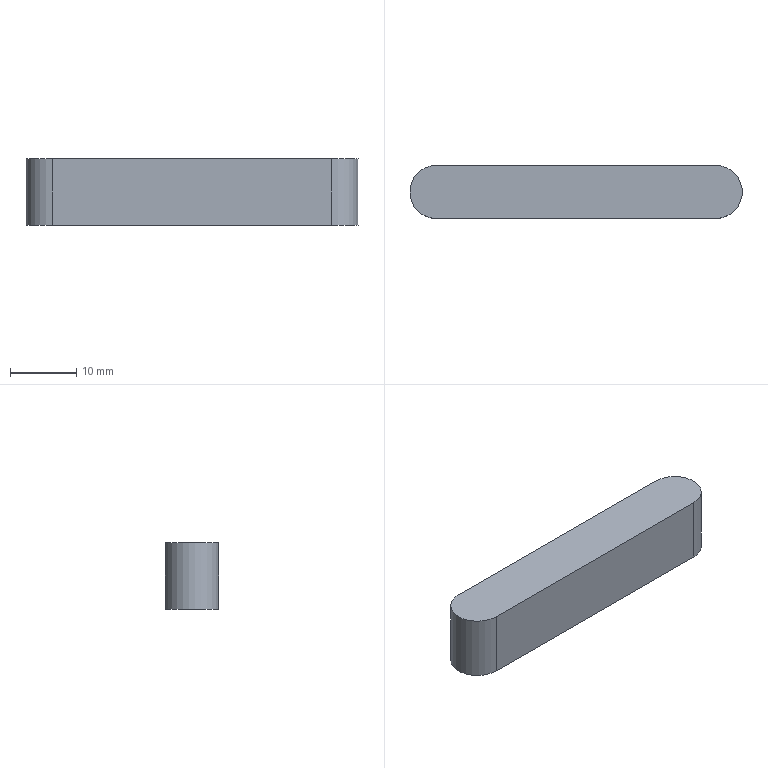Part | NX | features DATUM_CSYS 2, BLEND 1, EXTRUDE 1, SKETCH 1 | 1 solid | 6 faces | box 50 x 8 x 10 mm | volume 3863 mm3 | plane 4 | cylinder 2 | commonest cylinder face diameters 8 x2
STEP:
#1=CARTESIAN_POINT('',(-21.,-4.,10.));
#2=VERTEX_POINT('',#1);
#3=CARTESIAN_POINT('',(21.,-4.,10.));
#4=VERTEX_POINT('',#3);
#5=CARTESIAN_POINT('',(-25.,-4.,10.));
#6=DIRECTION('',(1.,0.,0.));
#7=VECTOR('',#6,1000.);
#8=LINE('',#5,#7);
#9=EDGE_CURVE('',#2,#4,#8,.T.);
#10=ORIENTED_EDGE('',*,*,#9,.F.);
#11=CARTESIAN_POINT('',(-21.,-4.,0.));
#12=VERTEX_POINT('',#11);
#13=CARTESIAN_POINT('',(-21.,-4.,10.));
#14=DIRECTION('',(0.,0.,-1.));
#15=VECTOR('',#14,1000.);
#16=LINE('',#13,#15);
#17=EDGE_CURVE('',#2,#12,#16,.T.);
#18=ORIENTED_EDGE('',*,*,#17,.T.);
#19=CARTESIAN_POINT('',(21.,-4.,0.));
#20=VERTEX_POINT('',#19);
#21=CARTESIAN_POINT('',(-25.,-4.,0.));
#22=DIRECTION('',(1.,0.,0.));
#23=VECTOR('',#22,1000.);
#24=LINE('',#21,#23);
#25=EDGE_CURVE('',#12,#20,#24,.T.);
#26=ORIENTED_EDGE('',*,*,#25,.T.);
#27=CARTESIAN_POINT('',(21.,-4.,10.));
#28=DIRECTION('',(0.,0.,-1.));
#29=VECTOR('',#28,1000.);
#30=LINE('',#27,#29);
#31=EDGE_CURVE('',#20,#4,#30,.F.);
#32=ORIENTED_EDGE('',*,*,#31,.T.);
#33=EDGE_LOOP('',(#10,#18,#26,#32));
#34=FACE_BOUND('',#33,.T.);
#35=CARTESIAN_POINT('',(-25.,-4.,10.));
#36=DIRECTION('',(0.,1.,0.));
#37=DIRECTION('',(0.,0.,1.));
#38=AXIS2_PLACEMENT_3D('',#35,#36,#37);
#39=PLANE('',#38);
#40=ADVANCED_FACE('',(#34),#39,.F.);
#41=CARTESIAN_POINT('',(21.,4.,0.));
#42=VERTEX_POINT('',#41);
#43=CARTESIAN_POINT('',(-21.,4.,0.));
#44=VERTEX_POINT('',#43);
#45=CARTESIAN_POINT('',(25.,4.,0.));
#46=DIRECTION('',(-1.,0.,0.));
#47=VECTOR('',#46,1000.);
#48=LINE('',#45,#47);
#49=EDGE_CURVE('',#42,#44,#48,.T.);
#50=ORIENTED_EDGE('',*,*,#49,.T.);
#51=CARTESIAN_POINT('',(-21.,4.,10.));
#52=VERTEX_POINT('',#51);
#53=CARTESIAN_POINT('',(-21.,4.,10.));
#54=DIRECTION('',(0.,0.,-1.));
#55=VECTOR('',#54,1000.);
#56=LINE('',#53,#55);
#57=EDGE_CURVE('',#44,#52,#56,.F.);
#58=ORIENTED_EDGE('',*,*,#57,.T.);
#59=CARTESIAN_POINT('',(21.,4.,10.));
#60=VERTEX_POINT('',#59);
#61=CARTESIAN_POINT('',(25.,4.,10.));
#62=DIRECTION('',(-1.,0.,0.));
#63=VECTOR('',#62,1000.);
#64=LINE('',#61,#63);
#65=EDGE_CURVE('',#60,#52,#64,.T.);
#66=ORIENTED_EDGE('',*,*,#65,.F.);
#67=CARTESIAN_POINT('',(21.,4.,10.));
#68=DIRECTION('',(0.,0.,-1.));
#69=VECTOR('',#68,1000.);
#70=LINE('',#67,#69);
#71=EDGE_CURVE('',#60,#42,#70,.T.);
#72=ORIENTED_EDGE('',*,*,#71,.T.);
#73=EDGE_LOOP('',(#50,#58,#66,#72));
#74=FACE_BOUND('',#73,.T.);
#75=CARTESIAN_POINT('',(25.,4.,10.));
#76=DIRECTION('',(0.,-1.,0.));
#77=DIRECTION('',(0.,0.,-1.));
#78=AXIS2_PLACEMENT_3D('',#75,#76,#77);
#79=PLANE('',#78);
#80=ADVANCED_FACE('',(#74),#79,.F.);
#81=ORIENTED_EDGE('',*,*,#65,.T.);
#82=CARTESIAN_POINT('',(-21.,0.,10.));
#83=DIRECTION('',(0.,0.,1.));
#84=DIRECTION('',(1.,0.,0.));
#85=AXIS2_PLACEMENT_3D('',#82,#83,#84);
#86=CIRCLE('',#85,4.);
#87=EDGE_CURVE('',#52,#2,#86,.T.);
#88=ORIENTED_EDGE('',*,*,#87,.T.);
#89=ORIENTED_EDGE('',*,*,#9,.T.);
#90=CARTESIAN_POINT('',(21.,0.,10.));
#91=DIRECTION('',(0.,0.,1.));
#92=DIRECTION('',(1.,0.,0.));
#93=AXIS2_PLACEMENT_3D('',#90,#91,#92);
#94=CIRCLE('',#93,4.);
#95=EDGE_CURVE('',#4,#60,#94,.T.);
#96=ORIENTED_EDGE('',*,*,#95,.T.);
#97=EDGE_LOOP('',(#81,#88,#89,#96));
#98=FACE_BOUND('',#97,.T.);
#99=CARTESIAN_POINT('',(0.,0.,10.));
#100=DIRECTION('',(0.,0.,1.));
#101=DIRECTION('',(1.,0.,0.));
#102=AXIS2_PLACEMENT_3D('',#99,#100,#101);
#103=PLANE('',#102);
#104=ADVANCED_FACE('',(#98),#103,.T.);
#105=CARTESIAN_POINT('',(-21.,0.,0.));
#106=DIRECTION('',(0.,0.,1.));
#107=DIRECTION('',(1.,0.,0.));
#108=AXIS2_PLACEMENT_3D('',#105,#106,#107);
#109=CIRCLE('',#108,4.);
#110=EDGE_CURVE('',#12,#44,#109,.F.);
#111=ORIENTED_EDGE('',*,*,#110,.T.);
#112=ORIENTED_EDGE('',*,*,#49,.F.);
#113=CARTESIAN_POINT('',(21.,0.,0.));
#114=DIRECTION('',(0.,0.,1.));
#115=DIRECTION('',(1.,0.,0.));
#116=AXIS2_PLACEMENT_3D('',#113,#114,#115);
#117=CIRCLE('',#116,4.);
#118=EDGE_CURVE('',#42,#20,#117,.F.);
#119=ORIENTED_EDGE('',*,*,#118,.T.);
#120=ORIENTED_EDGE('',*,*,#25,.F.);
#121=EDGE_LOOP('',(#111,#112,#119,#120));
#122=FACE_BOUND('',#121,.T.);
#123=CARTESIAN_POINT('',(0.,0.,0.));
#124=DIRECTION('',(0.,0.,1.));
#125=DIRECTION('',(1.,0.,0.));
#126=AXIS2_PLACEMENT_3D('',#123,#124,#125);
#127=PLANE('',#126);
#128=ADVANCED_FACE('',(#122),#127,.F.);
#129=ORIENTED_EDGE('',*,*,#17,.F.);
#130=ORIENTED_EDGE('',*,*,#87,.F.);
#131=ORIENTED_EDGE('',*,*,#57,.F.);
#132=ORIENTED_EDGE('',*,*,#110,.F.);
#133=EDGE_LOOP('',(#129,#130,#131,#132));
#134=FACE_BOUND('',#133,.T.);
#135=CARTESIAN_POINT('',(-21.,0.,10.));
#136=DIRECTION('',(0.,0.,-1.));
#137=DIRECTION('',(-1.,0.,0.));
#138=AXIS2_PLACEMENT_3D('',#135,#136,#137);
#139=CYLINDRICAL_SURFACE('',#138,4.);
#140=ADVANCED_FACE('',(#134),#139,.T.);
#141=ORIENTED_EDGE('',*,*,#118,.F.);
#142=ORIENTED_EDGE('',*,*,#71,.F.);
#143=ORIENTED_EDGE('',*,*,#95,.F.);
#144=ORIENTED_EDGE('',*,*,#31,.F.);
#145=EDGE_LOOP('',(#141,#142,#143,#144));
#146=FACE_BOUND('',#145,.T.);
#147=CARTESIAN_POINT('',(21.,0.,10.));
#148=DIRECTION('',(0.,0.,-1.));
#149=DIRECTION('',(-1.,0.,0.));
#150=AXIS2_PLACEMENT_3D('',#147,#148,#149);
#151=CYLINDRICAL_SURFACE('',#150,4.);
#152=ADVANCED_FACE('',(#146),#151,.T.);
#153=CLOSED_SHELL('',(#40,#80,#104,#128,#140,#152));
#154=MANIFOLD_SOLID_BREP('',#153);
#155=(LENGTH_UNIT()NAMED_UNIT(*)SI_UNIT(.MILLI.,.METRE.));
#156=UNCERTAINTY_MEASURE_WITH_UNIT(LENGTH_MEASURE(0.00001),#155,'','');
#157=(NAMED_UNIT(*)PLANE_ANGLE_UNIT()SI_UNIT($,.RADIAN.));
#158=(NAMED_UNIT(*)SI_UNIT($,.STERADIAN.)SOLID_ANGLE_UNIT());
#159=(GEOMETRIC_REPRESENTATION_CONTEXT(3)GLOBAL_UNCERTAINTY_ASSIGNED_CONTEXT((#156))GLOBAL_UNIT_ASSIGNED_CONTEXT((#155,#157,#158))REPRESENTATION_CONTEXT('',''));
#160=ADVANCED_BREP_SHAPE_REPRESENTATION('',(#154),#159);